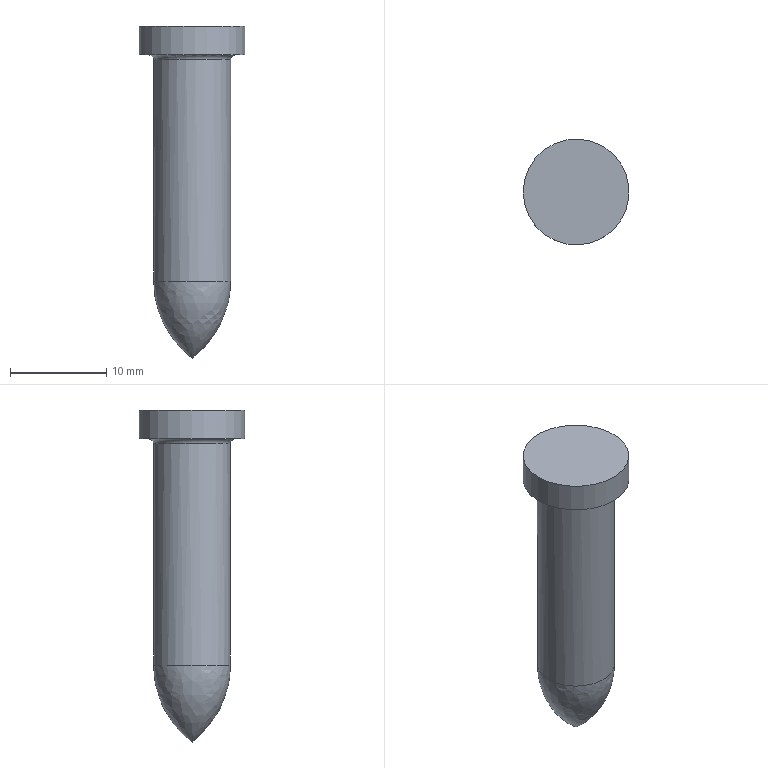Part | NX | features MI_SPT_0858 2 | 1 solid | 6 faces | box 11 x 11 x 34.5 mm | volume 1698 mm3 | cylinder 2 | plane 2 | torus 1 | spline 1 | commonest cylinder face diameters 8 x1 11 x1
STEP:
#1=CARTESIAN_POINT('',(-73.035,-84.,-1.5));
#2=VERTEX_POINT('',#1);
#3=CARTESIAN_POINT('',(-73.,-88.,-1.5));
#4=DIRECTION('',(0.,0.,-1.));
#5=DIRECTION('',(-1.,0.,0.));
#6=AXIS2_PLACEMENT_3D('',#3,#4,#5);
#7=CIRCLE('',#6,4.);
#8=EDGE_CURVE('',#2,#2,#7,.T.);
#9=ORIENTED_EDGE('',*,*,#8,.F.);
#10=EDGE_LOOP('',(#9));
#11=FACE_BOUND('',#10,.T.);
#12=CARTESIAN_POINT('',(-69.,-87.977,21.5));
#13=VERTEX_POINT('',#12);
#14=CARTESIAN_POINT('',(-73.,-88.,21.5));
#15=DIRECTION('',(0.,0.,1.));
#16=DIRECTION('',(-1.,0.,0.));
#17=AXIS2_PLACEMENT_3D('',#14,#15,#16);
#18=CIRCLE('',#17,4.);
#19=EDGE_CURVE('',#13,#13,#18,.T.);
#20=ORIENTED_EDGE('',*,*,#19,.F.);
#21=EDGE_LOOP('',(#20));
#22=FACE_BOUND('',#21,.T.);
#23=CARTESIAN_POINT('',(-73.,-88.,10.25));
#24=DIRECTION('',(0.,0.,-1.));
#25=DIRECTION('',(-0.008727,1.,0.));
#26=AXIS2_PLACEMENT_3D('',#23,#24,#25);
#27=CYLINDRICAL_SURFACE('',#26,4.);
#28=ADVANCED_FACE('',(#11,#22),#27,.T.);
#29=ORIENTED_EDGE('',*,*,#19,.T.);
#30=EDGE_LOOP('',(#29));
#31=FACE_BOUND('',#30,.T.);
#32=CARTESIAN_POINT('',(-68.5,-87.974,22.));
#33=VERTEX_POINT('',#32);
#34=CARTESIAN_POINT('',(-73.,-88.,22.));
#35=DIRECTION('',(0.,0.,-1.));
#36=DIRECTION('',(-1.,0.,0.));
#37=AXIS2_PLACEMENT_3D('',#34,#35,#36);
#38=CIRCLE('',#37,4.5);
#39=EDGE_CURVE('',#33,#33,#38,.T.);
#40=ORIENTED_EDGE('',*,*,#39,.T.);
#41=EDGE_LOOP('',(#40));
#42=FACE_BOUND('',#41,.T.);
#43=CARTESIAN_POINT('',(-73.,-88.,21.5));
#44=DIRECTION('',(0.,0.,1.));
#45=DIRECTION('',(1.,0.005818,0.));
#46=AXIS2_PLACEMENT_3D('',#43,#44,#45);
#47=TOROIDAL_SURFACE('',#46,4.5,0.5);
#48=ADVANCED_FACE('',(#31,#42),#47,.F.);
#49=CARTESIAN_POINT('',(-78.5,-88.,22.));
#50=VERTEX_POINT('',#49);
#51=CARTESIAN_POINT('',(-73.,-88.,22.));
#52=DIRECTION('',(0.,0.,-1.));
#53=DIRECTION('',(-1.,0.,0.));
#54=AXIS2_PLACEMENT_3D('',#51,#52,#53);
#55=CIRCLE('',#54,5.5);
#56=EDGE_CURVE('',#50,#50,#55,.T.);
#57=ORIENTED_EDGE('',*,*,#56,.T.);
#58=EDGE_LOOP('',(#57));
#59=FACE_BOUND('',#58,.T.);
#60=ORIENTED_EDGE('',*,*,#39,.F.);
#61=EDGE_LOOP('',(#60));
#62=FACE_BOUND('',#61,.T.);
#63=CARTESIAN_POINT('',(-60.35,-99.432,22.));
#64=DIRECTION('',(0.,0.,-1.));
#65=DIRECTION('',(-1.,0.,0.));
#66=AXIS2_PLACEMENT_3D('',#63,#64,#65);
#67=PLANE('',#66);
#68=ADVANCED_FACE('',(#59,#62),#67,.T.);
#69=CARTESIAN_POINT('',(-73.,-88.,-9.5));
#70=VERTEX_POINT('',#69);
#71=VERTEX_LOOP('',#70);
#72=FACE_BOUND('',#71,.T.);
#73=ORIENTED_EDGE('',*,*,#8,.T.);
#74=EDGE_LOOP('',(#73));
#75=FACE_BOUND('',#74,.T.);
#76=CARTESIAN_POINT('',(-77.,-88.,-1.5));
#77=CARTESIAN_POINT('',(-77.,-92.,-1.5));
#78=CARTESIAN_POINT('',(-73.,-92.,-1.5));
#79=CARTESIAN_POINT('',(-69.,-92.,-1.5));
#80=CARTESIAN_POINT('',(-69.,-88.,-1.5));
#81=CARTESIAN_POINT('',(-69.,-84.,-1.5));
#82=CARTESIAN_POINT('',(-73.,-84.,-1.5));
#83=CARTESIAN_POINT('',(-77.,-84.,-1.5));
#84=CARTESIAN_POINT('',(-77.,-88.,-1.5));
#85=CARTESIAN_POINT('',(-77.,-88.,-6.5));
#86=CARTESIAN_POINT('',(-77.,-92.,-6.5));
#87=CARTESIAN_POINT('',(-73.,-92.,-6.5));
#88=CARTESIAN_POINT('',(-69.,-92.,-6.5));
#89=CARTESIAN_POINT('',(-69.,-88.,-6.5));
#90=CARTESIAN_POINT('',(-69.,-84.,-6.5));
#91=CARTESIAN_POINT('',(-73.,-84.,-6.5));
#92=CARTESIAN_POINT('',(-77.,-84.,-6.5));
#93=CARTESIAN_POINT('',(-77.,-88.,-6.5));
#94=CARTESIAN_POINT('',(-73.,-88.,-9.5));
#95=CARTESIAN_POINT('',(-73.,-88.,-9.5));
#96=CARTESIAN_POINT('',(-73.,-88.,-9.5));
#97=CARTESIAN_POINT('',(-73.,-88.,-9.5));
#98=CARTESIAN_POINT('',(-73.,-88.,-9.5));
#99=CARTESIAN_POINT('',(-73.,-88.,-9.5));
#100=CARTESIAN_POINT('',(-73.,-88.,-9.5));
#101=CARTESIAN_POINT('',(-73.,-88.,-9.5));
#102=CARTESIAN_POINT('',(-73.,-88.,-9.5));
#103=(BOUNDED_SURFACE()B_SPLINE_SURFACE(2,2,((#76,#77,#78,#79,#80,#81,#82,#83,#84),(#85,#86,#87,#88,#89,#90,#91,#92,#93),(#94,#95,#96,#97,#98,#99,#100,#101,#102)),.TOROIDAL_SURF.,.F.,.T.,.F.)B_SPLINE_SURFACE_WITH_KNOTS((3,3),(3,2,2,2,3),(0.,0.9273),(0.,1.571,3.142,4.712,6.283),.PIECEWISE_BEZIER_KNOTS.)GEOMETRIC_REPRESENTATION_ITEM()RATIONAL_B_SPLINE_SURFACE(((1.,0.7071,1.,0.7071,1.,0.7071,1.,0.7071,1.),(0.8944,0.6325,0.8944,0.6325,0.8944,0.6325,0.8944,0.6325,0.8944),(1.,0.7071,1.,0.7071,1.,0.7071,1.,0.7071,1.)))REPRESENTATION_ITEM('')SURFACE());
#104=ADVANCED_FACE('',(#72,#75),#103,.T.);
#105=ORIENTED_EDGE('',*,*,#56,.F.);
#106=EDGE_LOOP('',(#105));
#107=FACE_BOUND('',#106,.T.);
#108=CARTESIAN_POINT('',(-78.5,-88.,25.));
#109=VERTEX_POINT('',#108);
#110=CARTESIAN_POINT('',(-73.,-88.,25.));
#111=DIRECTION('',(0.,0.,1.));
#112=DIRECTION('',(-1.,0.,0.));
#113=AXIS2_PLACEMENT_3D('',#110,#111,#112);
#114=CIRCLE('',#113,5.5);
#115=EDGE_CURVE('',#109,#109,#114,.T.);
#116=ORIENTED_EDGE('',*,*,#115,.F.);
#117=EDGE_LOOP('',(#116));
#118=FACE_BOUND('',#117,.T.);
#119=CARTESIAN_POINT('',(-73.,-88.,23.5));
#120=DIRECTION('',(0.,0.,-1.));
#121=DIRECTION('',(-1.,0.,0.));
#122=AXIS2_PLACEMENT_3D('',#119,#120,#121);
#123=CYLINDRICAL_SURFACE('',#122,5.5);
#124=ADVANCED_FACE('',(#107,#118),#123,.T.);
#125=ORIENTED_EDGE('',*,*,#115,.T.);
#126=EDGE_LOOP('',(#125));
#127=FACE_BOUND('',#126,.T.);
#128=CARTESIAN_POINT('',(-80.15,-99.432,25.));
#129=DIRECTION('',(0.,0.,1.));
#130=DIRECTION('',(1.,0.,0.));
#131=AXIS2_PLACEMENT_3D('',#128,#129,#130);
#132=PLANE('',#131);
#133=ADVANCED_FACE('',(#127),#132,.T.);
#134=CLOSED_SHELL('',(#28,#48,#68,#104,#124,#133));
#135=MANIFOLD_SOLID_BREP('',#134);
#136=(LENGTH_UNIT()NAMED_UNIT(*)SI_UNIT(.MILLI.,.METRE.));
#137=UNCERTAINTY_MEASURE_WITH_UNIT(LENGTH_MEASURE(0.00001),#136,'','');
#138=(NAMED_UNIT(*)PLANE_ANGLE_UNIT()SI_UNIT($,.RADIAN.));
#139=(NAMED_UNIT(*)SI_UNIT($,.STERADIAN.)SOLID_ANGLE_UNIT());
#140=(GEOMETRIC_REPRESENTATION_CONTEXT(3)GLOBAL_UNCERTAINTY_ASSIGNED_CONTEXT((#137))GLOBAL_UNIT_ASSIGNED_CONTEXT((#136,#138,#139))REPRESENTATION_CONTEXT('',''));
#141=ADVANCED_BREP_SHAPE_REPRESENTATION('',(#135),#140);